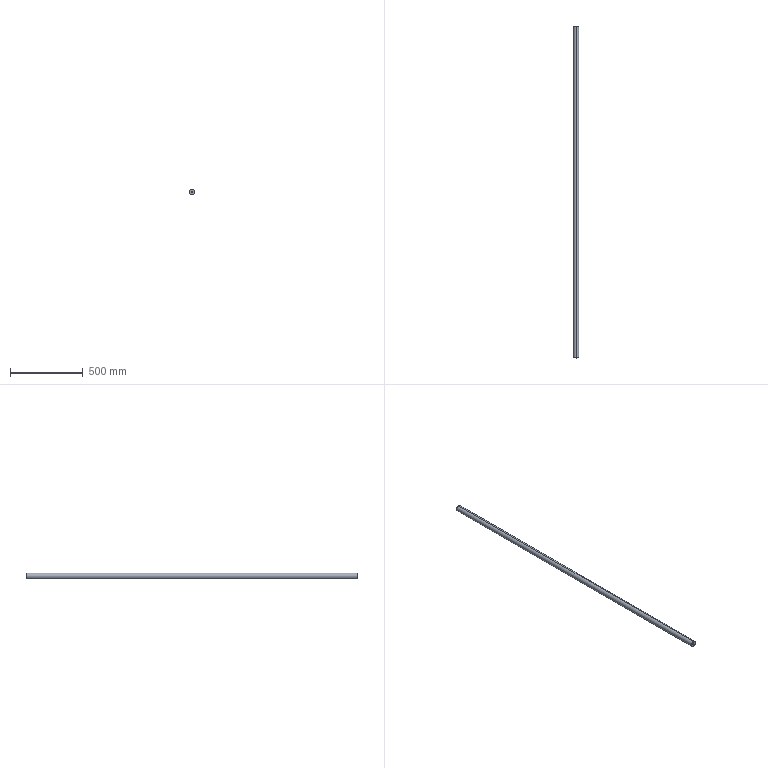Part | SolidWorks | features HoleWzd 2, Extrusion 1 | 1 solid | 12 faces | box 40 x 2286 x 40 mm | volume 2864710 mm3 | cylinder 6 | cone 4 | plane 2 | commonest cylinder face diameters 12 x4 40 x2
STEP:
#1=CARTESIAN_POINT('',(0.,34.,6.));
#2=VERTEX_POINT('',#1);
#3=CARTESIAN_POINT('',(0.,34.,-6.));
#4=VERTEX_POINT('',#3);
#5=CARTESIAN_POINT('',(0.,34.,0.));
#6=DIRECTION('',(0.,-1.,0.));
#7=DIRECTION('',(0.,0.,-1.));
#8=AXIS2_PLACEMENT_3D('',#5,#6,#7);
#9=CIRCLE('',#8,6.);
#10=EDGE_CURVE('',#2,#4,#9,.T.);
#11=ORIENTED_EDGE('',*,*,#10,.F.);
#12=CARTESIAN_POINT('',(0.,0.,6.));
#13=VERTEX_POINT('',#12);
#14=CARTESIAN_POINT('',(0.,0.,6.));
#15=DIRECTION('',(0.,-1.,0.));
#16=VECTOR('',#15,1000.);
#17=LINE('',#14,#16);
#18=EDGE_CURVE('',#2,#13,#17,.T.);
#19=ORIENTED_EDGE('',*,*,#18,.T.);
#20=CARTESIAN_POINT('',(0.,0.,-6.));
#21=VERTEX_POINT('',#20);
#22=CARTESIAN_POINT('',(0.,0.,0.));
#23=DIRECTION('',(0.,-1.,0.));
#24=DIRECTION('',(0.,0.,-1.));
#25=AXIS2_PLACEMENT_3D('',#22,#23,#24);
#26=CIRCLE('',#25,6.);
#27=EDGE_CURVE('',#13,#21,#26,.T.);
#28=ORIENTED_EDGE('',*,*,#27,.T.);
#29=CARTESIAN_POINT('',(0.,0.,-6.));
#30=DIRECTION('',(0.,-1.,0.));
#31=VECTOR('',#30,1000.);
#32=LINE('',#29,#31);
#33=EDGE_CURVE('',#4,#21,#32,.T.);
#34=ORIENTED_EDGE('',*,*,#33,.F.);
#35=EDGE_LOOP('',(#11,#19,#28,#34));
#36=FACE_OUTER_BOUND('',#35,.T.);
#37=CARTESIAN_POINT('',(0.,0.,0.));
#38=DIRECTION('',(0.,-1.,0.));
#39=DIRECTION('',(0.,0.,-1.));
#40=AXIS2_PLACEMENT_3D('',#37,#38,#39);
#41=CYLINDRICAL_SURFACE('',#40,6.);
#42=ADVANCED_FACE('',(#36),#41,.F.);
#43=CARTESIAN_POINT('',(0.,37.605,0.));
#44=VERTEX_POINT('',#43);
#45=CARTESIAN_POINT('',(0.,34.,-6.));
#46=DIRECTION('',(0.,-0.515,-0.8572));
#47=VECTOR('',#46,1000.);
#48=LINE('',#45,#47);
#49=EDGE_CURVE('',#44,#4,#48,.T.);
#50=ORIENTED_EDGE('',*,*,#49,.F.);
#51=CARTESIAN_POINT('',(0.,34.,6.));
#52=DIRECTION('',(0.,-0.515,0.8572));
#53=VECTOR('',#52,1000.);
#54=LINE('',#51,#53);
#55=EDGE_CURVE('',#44,#2,#54,.T.);
#56=ORIENTED_EDGE('',*,*,#55,.T.);
#57=ORIENTED_EDGE('',*,*,#10,.T.);
#58=EDGE_LOOP('',(#50,#56,#57));
#59=FACE_OUTER_BOUND('',#58,.T.);
#60=CARTESIAN_POINT('',(0.,34.,0.));
#61=DIRECTION('',(0.,-1.,0.));
#62=DIRECTION('',(0.,0.,-1.));
#63=AXIS2_PLACEMENT_3D('',#60,#61,#62);
#64=CONICAL_SURFACE('',#63,6.,1.03);
#65=ADVANCED_FACE('',(#59),#64,.F.);
#66=CARTESIAN_POINT('',(0.,2252.,-6.));
#67=VERTEX_POINT('',#66);
#68=CARTESIAN_POINT('',(0.,2252.,6.));
#69=VERTEX_POINT('',#68);
#70=CARTESIAN_POINT('',(0.,2252.,0.));
#71=DIRECTION('',(0.,1.,0.));
#72=DIRECTION('',(0.,0.,1.));
#73=AXIS2_PLACEMENT_3D('',#70,#71,#72);
#74=CIRCLE('',#73,6.);
#75=EDGE_CURVE('',#67,#69,#74,.T.);
#76=ORIENTED_EDGE('',*,*,#75,.F.);
#77=CARTESIAN_POINT('',(0.,2286.,-6.));
#78=VERTEX_POINT('',#77);
#79=CARTESIAN_POINT('',(0.,2286.,-6.));
#80=DIRECTION('',(0.,1.,0.));
#81=VECTOR('',#80,1000.);
#82=LINE('',#79,#81);
#83=EDGE_CURVE('',#67,#78,#82,.T.);
#84=ORIENTED_EDGE('',*,*,#83,.T.);
#85=CARTESIAN_POINT('',(0.,2286.,6.));
#86=VERTEX_POINT('',#85);
#87=CARTESIAN_POINT('',(0.,2286.,0.));
#88=DIRECTION('',(0.,1.,0.));
#89=DIRECTION('',(0.,0.,1.));
#90=AXIS2_PLACEMENT_3D('',#87,#88,#89);
#91=CIRCLE('',#90,6.);
#92=EDGE_CURVE('',#78,#86,#91,.T.);
#93=ORIENTED_EDGE('',*,*,#92,.T.);
#94=CARTESIAN_POINT('',(0.,2286.,6.));
#95=DIRECTION('',(0.,1.,0.));
#96=VECTOR('',#95,1000.);
#97=LINE('',#94,#96);
#98=EDGE_CURVE('',#69,#86,#97,.T.);
#99=ORIENTED_EDGE('',*,*,#98,.F.);
#100=EDGE_LOOP('',(#76,#84,#93,#99));
#101=FACE_OUTER_BOUND('',#100,.T.);
#102=CARTESIAN_POINT('',(0.,2286.,0.));
#103=DIRECTION('',(0.,1.,0.));
#104=DIRECTION('',(0.,0.,1.));
#105=AXIS2_PLACEMENT_3D('',#102,#103,#104);
#106=CYLINDRICAL_SURFACE('',#105,6.);
#107=ADVANCED_FACE('',(#101),#106,.F.);
#108=CARTESIAN_POINT('',(0.,2248.395,0.));
#109=VERTEX_POINT('',#108);
#110=CARTESIAN_POINT('',(0.,2252.,6.));
#111=DIRECTION('',(0.,0.515,0.8572));
#112=VECTOR('',#111,1000.);
#113=LINE('',#110,#112);
#114=EDGE_CURVE('',#109,#69,#113,.T.);
#115=ORIENTED_EDGE('',*,*,#114,.F.);
#116=CARTESIAN_POINT('',(0.,2252.,-6.));
#117=DIRECTION('',(0.,0.515,-0.8572));
#118=VECTOR('',#117,1000.);
#119=LINE('',#116,#118);
#120=EDGE_CURVE('',#109,#67,#119,.T.);
#121=ORIENTED_EDGE('',*,*,#120,.T.);
#122=ORIENTED_EDGE('',*,*,#75,.T.);
#123=EDGE_LOOP('',(#115,#121,#122));
#124=FACE_OUTER_BOUND('',#123,.T.);
#125=CARTESIAN_POINT('',(0.,2252.,0.));
#126=DIRECTION('',(0.,1.,0.));
#127=DIRECTION('',(0.,0.,1.));
#128=AXIS2_PLACEMENT_3D('',#125,#126,#127);
#129=CONICAL_SURFACE('',#128,6.,1.03);
#130=ADVANCED_FACE('',(#124),#129,.F.);
#131=CARTESIAN_POINT('',(0.,2286.,20.));
#132=VERTEX_POINT('',#131);
#133=CARTESIAN_POINT('',(0.,2286.,-20.));
#134=VERTEX_POINT('',#133);
#135=CARTESIAN_POINT('',(0.,2286.,0.));
#136=DIRECTION('',(0.,1.,0.));
#137=DIRECTION('',(0.,0.,1.));
#138=AXIS2_PLACEMENT_3D('',#135,#136,#137);
#139=CIRCLE('',#138,20.);
#140=EDGE_CURVE('',#132,#134,#139,.T.);
#141=ORIENTED_EDGE('',*,*,#140,.F.);
#142=CARTESIAN_POINT('',(0.,0.,20.));
#143=VERTEX_POINT('',#142);
#144=CARTESIAN_POINT('',(0.,2286.,20.));
#145=DIRECTION('',(0.,-1.,0.));
#146=VECTOR('',#145,1000.);
#147=LINE('',#144,#146);
#148=EDGE_CURVE('',#132,#143,#147,.T.);
#149=ORIENTED_EDGE('',*,*,#148,.T.);
#150=CARTESIAN_POINT('',(0.,0.,-20.));
#151=VERTEX_POINT('',#150);
#152=CARTESIAN_POINT('',(0.,0.,0.));
#153=DIRECTION('',(0.,1.,0.));
#154=DIRECTION('',(0.,0.,1.));
#155=AXIS2_PLACEMENT_3D('',#152,#153,#154);
#156=CIRCLE('',#155,20.);
#157=EDGE_CURVE('',#143,#151,#156,.T.);
#158=ORIENTED_EDGE('',*,*,#157,.T.);
#159=CARTESIAN_POINT('',(0.,2286.,-20.));
#160=DIRECTION('',(0.,-1.,0.));
#161=VECTOR('',#160,1000.);
#162=LINE('',#159,#161);
#163=EDGE_CURVE('',#134,#151,#162,.T.);
#164=ORIENTED_EDGE('',*,*,#163,.F.);
#165=EDGE_LOOP('',(#141,#149,#158,#164));
#166=FACE_OUTER_BOUND('',#165,.T.);
#167=CARTESIAN_POINT('',(0.,2286.,0.));
#168=DIRECTION('',(0.,-1.,0.));
#169=DIRECTION('',(0.,0.,-1.));
#170=AXIS2_PLACEMENT_3D('',#167,#168,#169);
#171=CYLINDRICAL_SURFACE('',#170,20.);
#172=ADVANCED_FACE('',(#166),#171,.T.);
#173=ORIENTED_EDGE('',*,*,#148,.F.);
#174=CARTESIAN_POINT('',(0.,2286.,0.));
#175=DIRECTION('',(0.,1.,0.));
#176=DIRECTION('',(0.,0.,1.));
#177=AXIS2_PLACEMENT_3D('',#174,#175,#176);
#178=CIRCLE('',#177,20.);
#179=EDGE_CURVE('',#134,#132,#178,.T.);
#180=ORIENTED_EDGE('',*,*,#179,.F.);
#181=ORIENTED_EDGE('',*,*,#163,.T.);
#182=CARTESIAN_POINT('',(0.,0.,0.));
#183=DIRECTION('',(0.,1.,0.));
#184=DIRECTION('',(0.,0.,1.));
#185=AXIS2_PLACEMENT_3D('',#182,#183,#184);
#186=CIRCLE('',#185,20.);
#187=EDGE_CURVE('',#151,#143,#186,.T.);
#188=ORIENTED_EDGE('',*,*,#187,.T.);
#189=EDGE_LOOP('',(#173,#180,#181,#188));
#190=FACE_OUTER_BOUND('',#189,.T.);
#191=CARTESIAN_POINT('',(0.,2286.,0.));
#192=DIRECTION('',(0.,-1.,0.));
#193=DIRECTION('',(0.,0.,-1.));
#194=AXIS2_PLACEMENT_3D('',#191,#192,#193);
#195=CYLINDRICAL_SURFACE('',#194,20.);
#196=ADVANCED_FACE('',(#190),#195,.T.);
#197=CARTESIAN_POINT('',(0.,2286.,0.));
#198=DIRECTION('',(0.,1.,0.));
#199=DIRECTION('',(0.,0.,1.));
#200=AXIS2_PLACEMENT_3D('',#197,#198,#199);
#201=CIRCLE('',#200,6.);
#202=EDGE_CURVE('',#86,#78,#201,.T.);
#203=ORIENTED_EDGE('',*,*,#202,.F.);
#204=ORIENTED_EDGE('',*,*,#92,.F.);
#205=EDGE_LOOP('',(#203,#204));
#206=FACE_BOUND('',#205,.T.);
#207=ORIENTED_EDGE('',*,*,#179,.T.);
#208=ORIENTED_EDGE('',*,*,#140,.T.);
#209=EDGE_LOOP('',(#207,#208));
#210=FACE_OUTER_BOUND('',#209,.T.);
#211=CARTESIAN_POINT('',(0.,2286.,0.));
#212=DIRECTION('',(0.,1.,0.));
#213=DIRECTION('',(0.,0.,1.));
#214=AXIS2_PLACEMENT_3D('',#211,#212,#213);
#215=PLANE('',#214);
#216=ADVANCED_FACE('',(#206,#210),#215,.T.);
#217=CARTESIAN_POINT('',(0.,0.,0.));
#218=DIRECTION('',(0.,-1.,0.));
#219=DIRECTION('',(0.,0.,-1.));
#220=AXIS2_PLACEMENT_3D('',#217,#218,#219);
#221=CIRCLE('',#220,6.);
#222=EDGE_CURVE('',#21,#13,#221,.T.);
#223=ORIENTED_EDGE('',*,*,#222,.F.);
#224=ORIENTED_EDGE('',*,*,#27,.F.);
#225=EDGE_LOOP('',(#223,#224));
#226=FACE_BOUND('',#225,.T.);
#227=ORIENTED_EDGE('',*,*,#187,.F.);
#228=ORIENTED_EDGE('',*,*,#157,.F.);
#229=EDGE_LOOP('',(#227,#228));
#230=FACE_OUTER_BOUND('',#229,.T.);
#231=CARTESIAN_POINT('',(0.,0.,0.));
#232=DIRECTION('',(0.,1.,0.));
#233=DIRECTION('',(0.,0.,1.));
#234=AXIS2_PLACEMENT_3D('',#231,#232,#233);
#235=PLANE('',#234);
#236=ADVANCED_FACE('',(#226,#230),#235,.F.);
#237=ORIENTED_EDGE('',*,*,#120,.F.);
#238=ORIENTED_EDGE('',*,*,#114,.T.);
#239=CARTESIAN_POINT('',(0.,2252.,0.));
#240=DIRECTION('',(0.,1.,0.));
#241=DIRECTION('',(0.,0.,1.));
#242=AXIS2_PLACEMENT_3D('',#239,#240,#241);
#243=CIRCLE('',#242,6.);
#244=EDGE_CURVE('',#69,#67,#243,.T.);
#245=ORIENTED_EDGE('',*,*,#244,.T.);
#246=EDGE_LOOP('',(#237,#238,#245));
#247=FACE_OUTER_BOUND('',#246,.T.);
#248=CARTESIAN_POINT('',(0.,2252.,0.));
#249=DIRECTION('',(0.,1.,0.));
#250=DIRECTION('',(0.,0.,1.));
#251=AXIS2_PLACEMENT_3D('',#248,#249,#250);
#252=CONICAL_SURFACE('',#251,6.,1.03);
#253=ADVANCED_FACE('',(#247),#252,.F.);
#254=ORIENTED_EDGE('',*,*,#83,.F.);
#255=ORIENTED_EDGE('',*,*,#244,.F.);
#256=ORIENTED_EDGE('',*,*,#98,.T.);
#257=ORIENTED_EDGE('',*,*,#202,.T.);
#258=EDGE_LOOP('',(#254,#255,#256,#257));
#259=FACE_OUTER_BOUND('',#258,.T.);
#260=CARTESIAN_POINT('',(0.,2286.,0.));
#261=DIRECTION('',(0.,1.,0.));
#262=DIRECTION('',(0.,0.,1.));
#263=AXIS2_PLACEMENT_3D('',#260,#261,#262);
#264=CYLINDRICAL_SURFACE('',#263,6.);
#265=ADVANCED_FACE('',(#259),#264,.F.);
#266=ORIENTED_EDGE('',*,*,#55,.F.);
#267=ORIENTED_EDGE('',*,*,#49,.T.);
#268=CARTESIAN_POINT('',(0.,34.,0.));
#269=DIRECTION('',(0.,-1.,0.));
#270=DIRECTION('',(0.,0.,-1.));
#271=AXIS2_PLACEMENT_3D('',#268,#269,#270);
#272=CIRCLE('',#271,6.);
#273=EDGE_CURVE('',#4,#2,#272,.T.);
#274=ORIENTED_EDGE('',*,*,#273,.T.);
#275=EDGE_LOOP('',(#266,#267,#274));
#276=FACE_OUTER_BOUND('',#275,.T.);
#277=CARTESIAN_POINT('',(0.,34.,0.));
#278=DIRECTION('',(0.,-1.,0.));
#279=DIRECTION('',(0.,0.,-1.));
#280=AXIS2_PLACEMENT_3D('',#277,#278,#279);
#281=CONICAL_SURFACE('',#280,6.,1.03);
#282=ADVANCED_FACE('',(#276),#281,.F.);
#283=ORIENTED_EDGE('',*,*,#18,.F.);
#284=ORIENTED_EDGE('',*,*,#273,.F.);
#285=ORIENTED_EDGE('',*,*,#33,.T.);
#286=ORIENTED_EDGE('',*,*,#222,.T.);
#287=EDGE_LOOP('',(#283,#284,#285,#286));
#288=FACE_OUTER_BOUND('',#287,.T.);
#289=CARTESIAN_POINT('',(0.,0.,0.));
#290=DIRECTION('',(0.,-1.,0.));
#291=DIRECTION('',(0.,0.,-1.));
#292=AXIS2_PLACEMENT_3D('',#289,#290,#291);
#293=CYLINDRICAL_SURFACE('',#292,6.);
#294=ADVANCED_FACE('',(#288),#293,.F.);
#295=CLOSED_SHELL('',(#42,#65,#107,#130,#172,#196,#216,#236,#253,#265,#282,#294));
#296=MANIFOLD_SOLID_BREP('',#295);
#297=CARTESIAN_POINT('',(0.,0.,0.));
#298=DIRECTION('',(0.,0.,1.));
#299=DIRECTION('',(1.,0.,0.));
#300=AXIS2_PLACEMENT_3D('',#297,#298,#299);
#301=(LENGTH_UNIT()NAMED_UNIT(*)SI_UNIT(.MILLI.,.METRE.));
#302=UNCERTAINTY_MEASURE_WITH_UNIT(LENGTH_MEASURE(0.00001),#301,'','');
#303=(NAMED_UNIT(*)PLANE_ANGLE_UNIT()SI_UNIT($,.RADIAN.));
#304=(NAMED_UNIT(*)SI_UNIT($,.STERADIAN.)SOLID_ANGLE_UNIT());
#305=(GEOMETRIC_REPRESENTATION_CONTEXT(3)GLOBAL_UNCERTAINTY_ASSIGNED_CONTEXT((#302))GLOBAL_UNIT_ASSIGNED_CONTEXT((#301,#303,#304))REPRESENTATION_CONTEXT('',''));
#306=ADVANCED_BREP_SHAPE_REPRESENTATION('',(#296,#300),#305);